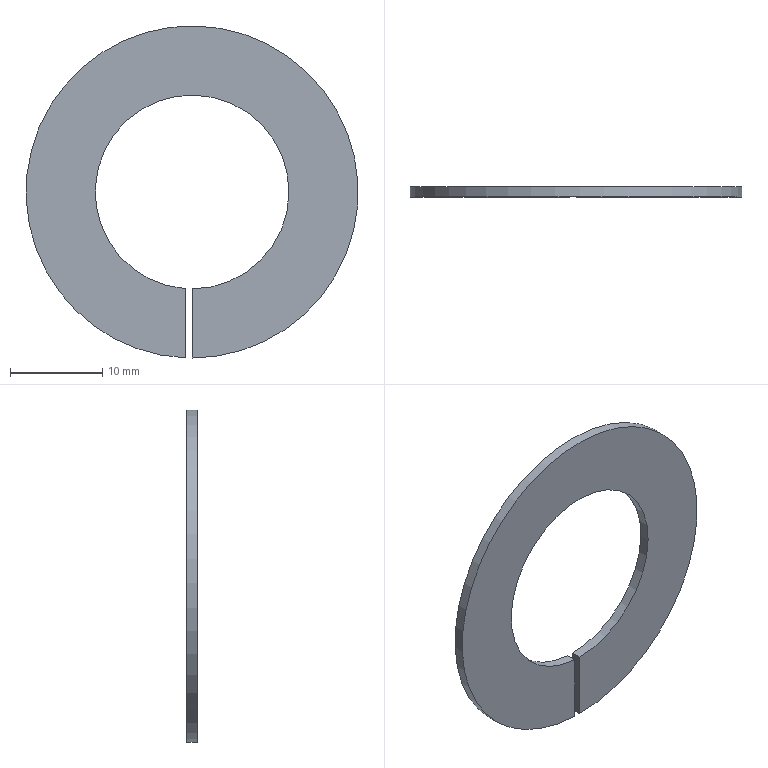Part | SolidWorks | features Extrusion 1 | 1 solid | 6 faces | box 36 x 1.1 x 36 mm | volume 732.535 mm3 | plane 4 | cylinder 2 | commonest cylinder face diameters 21 x1 36 x1
STEP:
#1=CARTESIAN_POINT('',(0.,0.,-10.5));
#2=VERTEX_POINT('',#1);
#3=CARTESIAN_POINT('',(-0.7429,0.,-10.474));
#4=VERTEX_POINT('',#3);
#5=CARTESIAN_POINT('',(0.,0.,0.));
#6=DIRECTION('',(0.,-1.,0.));
#7=DIRECTION('',(0.,0.,1.));
#8=AXIS2_PLACEMENT_3D('',#5,#6,#7);
#9=CIRCLE('',#8,10.5);
#10=EDGE_CURVE('',#2,#4,#9,.T.);
#11=ORIENTED_EDGE('',*,*,#10,.T.);
#12=CARTESIAN_POINT('',(-0.7429,1.1,-10.474));
#13=VERTEX_POINT('',#12);
#14=CARTESIAN_POINT('',(-0.7429,1.1,-10.474));
#15=DIRECTION('',(0.,-1.,0.));
#16=VECTOR('',#15,1000.);
#17=LINE('',#14,#16);
#18=EDGE_CURVE('',#13,#4,#17,.T.);
#19=ORIENTED_EDGE('',*,*,#18,.F.);
#20=CARTESIAN_POINT('',(0.,1.1,-10.5));
#21=VERTEX_POINT('',#20);
#22=CARTESIAN_POINT('',(0.,1.1,0.));
#23=DIRECTION('',(0.,-1.,0.));
#24=DIRECTION('',(0.,0.,1.));
#25=AXIS2_PLACEMENT_3D('',#22,#23,#24);
#26=CIRCLE('',#25,10.5);
#27=EDGE_CURVE('',#21,#13,#26,.T.);
#28=ORIENTED_EDGE('',*,*,#27,.F.);
#29=CARTESIAN_POINT('',(0.,1.1,-10.5));
#30=DIRECTION('',(0.,-1.,0.));
#31=VECTOR('',#30,1000.);
#32=LINE('',#29,#31);
#33=EDGE_CURVE('',#21,#2,#32,.T.);
#34=ORIENTED_EDGE('',*,*,#33,.T.);
#35=EDGE_LOOP('',(#11,#19,#28,#34));
#36=FACE_OUTER_BOUND('',#35,.T.);
#37=CARTESIAN_POINT('',(0.,1.1,0.));
#38=DIRECTION('',(0.,-1.,0.));
#39=DIRECTION('',(0.,0.,-1.));
#40=AXIS2_PLACEMENT_3D('',#37,#38,#39);
#41=CYLINDRICAL_SURFACE('',#40,10.5);
#42=ADVANCED_FACE('',(#36),#41,.F.);
#43=CARTESIAN_POINT('',(-0.7429,0.,-17.985));
#44=VERTEX_POINT('',#43);
#45=CARTESIAN_POINT('',(-0.7429,0.,-17.985));
#46=DIRECTION('',(0.,0.,-1.));
#47=VECTOR('',#46,1000.);
#48=LINE('',#45,#47);
#49=EDGE_CURVE('',#4,#44,#48,.T.);
#50=ORIENTED_EDGE('',*,*,#49,.T.);
#51=CARTESIAN_POINT('',(-0.7429,1.1,-17.985));
#52=VERTEX_POINT('',#51);
#53=CARTESIAN_POINT('',(-0.7429,1.1,-17.985));
#54=DIRECTION('',(0.,-1.,0.));
#55=VECTOR('',#54,1000.);
#56=LINE('',#53,#55);
#57=EDGE_CURVE('',#52,#44,#56,.T.);
#58=ORIENTED_EDGE('',*,*,#57,.F.);
#59=CARTESIAN_POINT('',(-0.7429,1.1,-17.985));
#60=DIRECTION('',(0.,0.,-1.));
#61=VECTOR('',#60,1000.);
#62=LINE('',#59,#61);
#63=EDGE_CURVE('',#13,#52,#62,.T.);
#64=ORIENTED_EDGE('',*,*,#63,.F.);
#65=ORIENTED_EDGE('',*,*,#18,.T.);
#66=EDGE_LOOP('',(#50,#58,#64,#65));
#67=FACE_OUTER_BOUND('',#66,.T.);
#68=CARTESIAN_POINT('',(-0.7429,1.1,-17.985));
#69=DIRECTION('',(-1.,0.,0.));
#70=DIRECTION('',(0.,0.,1.));
#71=AXIS2_PLACEMENT_3D('',#68,#69,#70);
#72=PLANE('',#71);
#73=ADVANCED_FACE('',(#67),#72,.F.);
#74=CARTESIAN_POINT('',(0.,0.,-18.));
#75=VERTEX_POINT('',#74);
#76=CARTESIAN_POINT('',(0.,0.,0.));
#77=DIRECTION('',(0.,1.,0.));
#78=DIRECTION('',(0.,0.,1.));
#79=AXIS2_PLACEMENT_3D('',#76,#77,#78);
#80=CIRCLE('',#79,18.);
#81=EDGE_CURVE('',#44,#75,#80,.T.);
#82=ORIENTED_EDGE('',*,*,#81,.T.);
#83=CARTESIAN_POINT('',(0.,1.1,-18.));
#84=VERTEX_POINT('',#83);
#85=CARTESIAN_POINT('',(0.,1.1,-18.));
#86=DIRECTION('',(0.,-1.,0.));
#87=VECTOR('',#86,1000.);
#88=LINE('',#85,#87);
#89=EDGE_CURVE('',#84,#75,#88,.T.);
#90=ORIENTED_EDGE('',*,*,#89,.F.);
#91=CARTESIAN_POINT('',(0.,1.1,0.));
#92=DIRECTION('',(0.,1.,0.));
#93=DIRECTION('',(0.,0.,1.));
#94=AXIS2_PLACEMENT_3D('',#91,#92,#93);
#95=CIRCLE('',#94,18.);
#96=EDGE_CURVE('',#52,#84,#95,.T.);
#97=ORIENTED_EDGE('',*,*,#96,.F.);
#98=ORIENTED_EDGE('',*,*,#57,.T.);
#99=EDGE_LOOP('',(#82,#90,#97,#98));
#100=FACE_OUTER_BOUND('',#99,.T.);
#101=CARTESIAN_POINT('',(0.,1.1,0.));
#102=DIRECTION('',(0.,-1.,0.));
#103=DIRECTION('',(0.,0.,-1.));
#104=AXIS2_PLACEMENT_3D('',#101,#102,#103);
#105=CYLINDRICAL_SURFACE('',#104,18.);
#106=ADVANCED_FACE('',(#100),#105,.T.);
#107=CARTESIAN_POINT('',(0.,0.,-10.5));
#108=DIRECTION('',(0.,0.,1.));
#109=VECTOR('',#108,1000.);
#110=LINE('',#107,#109);
#111=EDGE_CURVE('',#75,#2,#110,.T.);
#112=ORIENTED_EDGE('',*,*,#111,.T.);
#113=ORIENTED_EDGE('',*,*,#33,.F.);
#114=CARTESIAN_POINT('',(0.,1.1,-10.5));
#115=DIRECTION('',(0.,0.,1.));
#116=VECTOR('',#115,1000.);
#117=LINE('',#114,#116);
#118=EDGE_CURVE('',#84,#21,#117,.T.);
#119=ORIENTED_EDGE('',*,*,#118,.F.);
#120=ORIENTED_EDGE('',*,*,#89,.T.);
#121=EDGE_LOOP('',(#112,#113,#119,#120));
#122=FACE_OUTER_BOUND('',#121,.T.);
#123=CARTESIAN_POINT('',(0.,1.1,-10.5));
#124=DIRECTION('',(1.,0.,0.));
#125=DIRECTION('',(0.,0.,-1.));
#126=AXIS2_PLACEMENT_3D('',#123,#124,#125);
#127=PLANE('',#126);
#128=ADVANCED_FACE('',(#122),#127,.F.);
#129=ORIENTED_EDGE('',*,*,#27,.T.);
#130=ORIENTED_EDGE('',*,*,#63,.T.);
#131=ORIENTED_EDGE('',*,*,#96,.T.);
#132=ORIENTED_EDGE('',*,*,#118,.T.);
#133=EDGE_LOOP('',(#129,#130,#131,#132));
#134=FACE_OUTER_BOUND('',#133,.T.);
#135=CARTESIAN_POINT('',(0.,1.1,0.));
#136=DIRECTION('',(0.,1.,0.));
#137=DIRECTION('',(0.,0.,1.));
#138=AXIS2_PLACEMENT_3D('',#135,#136,#137);
#139=PLANE('',#138);
#140=ADVANCED_FACE('',(#134),#139,.T.);
#141=ORIENTED_EDGE('',*,*,#10,.F.);
#142=ORIENTED_EDGE('',*,*,#111,.F.);
#143=ORIENTED_EDGE('',*,*,#81,.F.);
#144=ORIENTED_EDGE('',*,*,#49,.F.);
#145=EDGE_LOOP('',(#141,#142,#143,#144));
#146=FACE_OUTER_BOUND('',#145,.T.);
#147=CARTESIAN_POINT('',(0.,0.,0.));
#148=DIRECTION('',(0.,1.,0.));
#149=DIRECTION('',(0.,0.,1.));
#150=AXIS2_PLACEMENT_3D('',#147,#148,#149);
#151=PLANE('',#150);
#152=ADVANCED_FACE('',(#146),#151,.F.);
#153=CLOSED_SHELL('',(#42,#73,#106,#128,#140,#152));
#154=MANIFOLD_SOLID_BREP('',#153);
#155=CARTESIAN_POINT('',(0.,0.,0.));
#156=DIRECTION('',(0.,0.,1.));
#157=DIRECTION('',(1.,0.,0.));
#158=AXIS2_PLACEMENT_3D('',#155,#156,#157);
#159=(LENGTH_UNIT()NAMED_UNIT(*)SI_UNIT(.MILLI.,.METRE.));
#160=UNCERTAINTY_MEASURE_WITH_UNIT(LENGTH_MEASURE(0.00001),#159,'','');
#161=(NAMED_UNIT(*)PLANE_ANGLE_UNIT()SI_UNIT($,.RADIAN.));
#162=(NAMED_UNIT(*)SI_UNIT($,.STERADIAN.)SOLID_ANGLE_UNIT());
#163=(GEOMETRIC_REPRESENTATION_CONTEXT(3)GLOBAL_UNCERTAINTY_ASSIGNED_CONTEXT((#160))GLOBAL_UNIT_ASSIGNED_CONTEXT((#159,#161,#162))REPRESENTATION_CONTEXT('',''));
#164=ADVANCED_BREP_SHAPE_REPRESENTATION('',(#154,#158),#163);